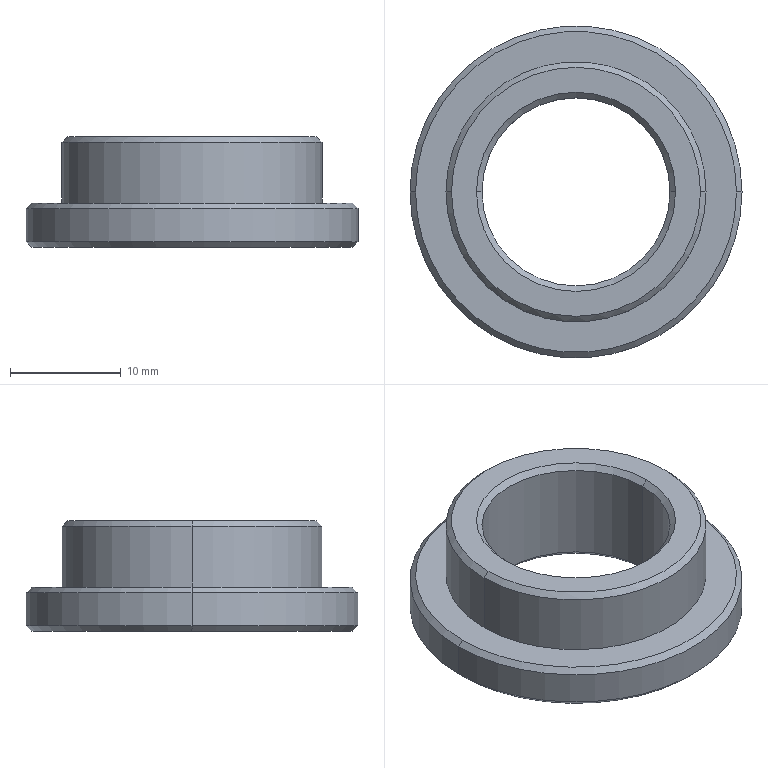Part | SolidWorks | features Chamfer 2, ICE 2, Extrusion 1 | 1 solid | 19 faces | box 30 x 30 x 10 mm | volume 3114 mm3 | cone 10 | cylinder 6 | plane 3 | commonest cylinder face diameters 17 x2 23.5 x2 30 x2
STEP:
#1=CARTESIAN_POINT('',(11.25,0.,10.));
#2=VERTEX_POINT('',#1);
#3=CARTESIAN_POINT('',(-11.25,0.,10.));
#4=VERTEX_POINT('',#3);
#5=CARTESIAN_POINT('',(0.,0.,10.));
#6=DIRECTION('',(0.,0.,1.));
#7=DIRECTION('',(1.,0.,0.));
#8=AXIS2_PLACEMENT_3D('',#5,#6,#7);
#9=CIRCLE('',#8,11.25);
#10=EDGE_CURVE('',#2,#4,#9,.T.);
#11=ORIENTED_EDGE('',*,*,#10,.F.);
#12=CARTESIAN_POINT('',(11.75,0.,9.5));
#13=VERTEX_POINT('',#12);
#14=CARTESIAN_POINT('',(11.25,0.,10.));
#15=DIRECTION('',(0.7071,0.,-0.7071));
#16=VECTOR('',#15,1000.);
#17=LINE('',#14,#16);
#18=EDGE_CURVE('',#2,#13,#17,.T.);
#19=ORIENTED_EDGE('',*,*,#18,.T.);
#20=CARTESIAN_POINT('',(-11.75,0.,9.5));
#21=VERTEX_POINT('',#20);
#22=CARTESIAN_POINT('',(0.,0.,9.5));
#23=DIRECTION('',(0.,0.,-1.));
#24=DIRECTION('',(1.,0.,0.));
#25=AXIS2_PLACEMENT_3D('',#22,#23,#24);
#26=CIRCLE('',#25,11.75);
#27=EDGE_CURVE('',#21,#13,#26,.T.);
#28=ORIENTED_EDGE('',*,*,#27,.F.);
#29=CARTESIAN_POINT('',(-11.25,0.,10.));
#30=DIRECTION('',(-0.7071,0.,-0.7071));
#31=VECTOR('',#30,1000.);
#32=LINE('',#29,#31);
#33=EDGE_CURVE('',#4,#21,#32,.T.);
#34=ORIENTED_EDGE('',*,*,#33,.F.);
#35=EDGE_LOOP('',(#11,#19,#28,#34));
#36=FACE_OUTER_BOUND('',#35,.T.);
#37=CARTESIAN_POINT('',(0.,0.,10.));
#38=DIRECTION('',(0.,0.,-1.));
#39=DIRECTION('',(-1.,0.,0.));
#40=AXIS2_PLACEMENT_3D('',#37,#38,#39);
#41=CONICAL_SURFACE('',#40,11.25,0.7854);
#42=ADVANCED_FACE('',(#36),#41,.T.);
#43=CARTESIAN_POINT('',(14.5,0.,4.));
#44=VERTEX_POINT('',#43);
#45=CARTESIAN_POINT('',(-14.5,0.,4.));
#46=VERTEX_POINT('',#45);
#47=CARTESIAN_POINT('',(0.,0.,4.));
#48=DIRECTION('',(0.,0.,1.));
#49=DIRECTION('',(1.,0.,0.));
#50=AXIS2_PLACEMENT_3D('',#47,#48,#49);
#51=CIRCLE('',#50,14.5);
#52=EDGE_CURVE('',#44,#46,#51,.T.);
#53=ORIENTED_EDGE('',*,*,#52,.F.);
#54=CARTESIAN_POINT('',(15.,0.,3.5));
#55=VERTEX_POINT('',#54);
#56=CARTESIAN_POINT('',(14.5,0.,4.));
#57=DIRECTION('',(0.7071,0.,-0.7071));
#58=VECTOR('',#57,1000.);
#59=LINE('',#56,#58);
#60=EDGE_CURVE('',#44,#55,#59,.T.);
#61=ORIENTED_EDGE('',*,*,#60,.T.);
#62=CARTESIAN_POINT('',(-15.,0.,3.5));
#63=VERTEX_POINT('',#62);
#64=CARTESIAN_POINT('',(0.,0.,3.5));
#65=DIRECTION('',(0.,0.,-1.));
#66=DIRECTION('',(1.,0.,0.));
#67=AXIS2_PLACEMENT_3D('',#64,#65,#66);
#68=CIRCLE('',#67,15.);
#69=EDGE_CURVE('',#63,#55,#68,.T.);
#70=ORIENTED_EDGE('',*,*,#69,.F.);
#71=CARTESIAN_POINT('',(-14.5,0.,4.));
#72=DIRECTION('',(-0.7071,0.,-0.7071));
#73=VECTOR('',#72,1000.);
#74=LINE('',#71,#73);
#75=EDGE_CURVE('',#46,#63,#74,.T.);
#76=ORIENTED_EDGE('',*,*,#75,.F.);
#77=EDGE_LOOP('',(#53,#61,#70,#76));
#78=FACE_OUTER_BOUND('',#77,.T.);
#79=CARTESIAN_POINT('',(0.,0.,4.));
#80=DIRECTION('',(0.,0.,-1.));
#81=DIRECTION('',(-1.,0.,0.));
#82=AXIS2_PLACEMENT_3D('',#79,#80,#81);
#83=CONICAL_SURFACE('',#82,14.5,0.7854);
#84=ADVANCED_FACE('',(#78),#83,.T.);
#85=CARTESIAN_POINT('',(-14.5,0.,0.));
#86=VERTEX_POINT('',#85);
#87=CARTESIAN_POINT('',(14.5,0.,0.));
#88=VERTEX_POINT('',#87);
#89=CARTESIAN_POINT('',(0.,0.,0.));
#90=DIRECTION('',(0.,0.,-1.));
#91=DIRECTION('',(1.,0.,0.));
#92=AXIS2_PLACEMENT_3D('',#89,#90,#91);
#93=CIRCLE('',#92,14.5);
#94=EDGE_CURVE('',#86,#88,#93,.T.);
#95=ORIENTED_EDGE('',*,*,#94,.F.);
#96=CARTESIAN_POINT('',(-15.,0.,0.5));
#97=VERTEX_POINT('',#96);
#98=CARTESIAN_POINT('',(-15.,0.,0.5));
#99=DIRECTION('',(-0.7071,0.,0.7071));
#100=VECTOR('',#99,1000.);
#101=LINE('',#98,#100);
#102=EDGE_CURVE('',#86,#97,#101,.T.);
#103=ORIENTED_EDGE('',*,*,#102,.T.);
#104=CARTESIAN_POINT('',(15.,0.,0.5));
#105=VERTEX_POINT('',#104);
#106=CARTESIAN_POINT('',(0.,0.,0.5));
#107=DIRECTION('',(0.,0.,1.));
#108=DIRECTION('',(1.,0.,0.));
#109=AXIS2_PLACEMENT_3D('',#106,#107,#108);
#110=CIRCLE('',#109,15.);
#111=EDGE_CURVE('',#105,#97,#110,.T.);
#112=ORIENTED_EDGE('',*,*,#111,.F.);
#113=CARTESIAN_POINT('',(15.,0.,0.5));
#114=DIRECTION('',(0.7071,0.,0.7071));
#115=VECTOR('',#114,1000.);
#116=LINE('',#113,#115);
#117=EDGE_CURVE('',#88,#105,#116,.T.);
#118=ORIENTED_EDGE('',*,*,#117,.F.);
#119=EDGE_LOOP('',(#95,#103,#112,#118));
#120=FACE_OUTER_BOUND('',#119,.T.);
#121=CARTESIAN_POINT('',(0.,0.,0.5));
#122=DIRECTION('',(0.,0.,1.));
#123=DIRECTION('',(1.,0.,0.));
#124=AXIS2_PLACEMENT_3D('',#121,#122,#123);
#125=CONICAL_SURFACE('',#124,15.,0.7854);
#126=ADVANCED_FACE('',(#120),#125,.T.);
#127=CARTESIAN_POINT('',(-8.5,0.,9.5));
#128=VERTEX_POINT('',#127);
#129=CARTESIAN_POINT('',(8.5,0.,9.5));
#130=VERTEX_POINT('',#129);
#131=CARTESIAN_POINT('',(0.,0.,9.5));
#132=DIRECTION('',(0.,0.,1.));
#133=DIRECTION('',(1.,0.,0.));
#134=AXIS2_PLACEMENT_3D('',#131,#132,#133);
#135=CIRCLE('',#134,8.5);
#136=EDGE_CURVE('',#128,#130,#135,.T.);
#137=ORIENTED_EDGE('',*,*,#136,.F.);
#138=CARTESIAN_POINT('',(-9.,0.,10.));
#139=VERTEX_POINT('',#138);
#140=CARTESIAN_POINT('',(-8.5,0.,9.5));
#141=DIRECTION('',(-0.7071,0.,0.7071));
#142=VECTOR('',#141,1000.);
#143=LINE('',#140,#142);
#144=EDGE_CURVE('',#128,#139,#143,.T.);
#145=ORIENTED_EDGE('',*,*,#144,.T.);
#146=CARTESIAN_POINT('',(9.,0.,10.));
#147=VERTEX_POINT('',#146);
#148=CARTESIAN_POINT('',(0.,0.,10.));
#149=DIRECTION('',(0.,0.,-1.));
#150=DIRECTION('',(1.,0.,0.));
#151=AXIS2_PLACEMENT_3D('',#148,#149,#150);
#152=CIRCLE('',#151,9.);
#153=EDGE_CURVE('',#147,#139,#152,.T.);
#154=ORIENTED_EDGE('',*,*,#153,.F.);
#155=CARTESIAN_POINT('',(8.5,0.,9.5));
#156=DIRECTION('',(0.7071,0.,0.7071));
#157=VECTOR('',#156,1000.);
#158=LINE('',#155,#157);
#159=EDGE_CURVE('',#130,#147,#158,.T.);
#160=ORIENTED_EDGE('',*,*,#159,.F.);
#161=EDGE_LOOP('',(#137,#145,#154,#160));
#162=FACE_OUTER_BOUND('',#161,.T.);
#163=CARTESIAN_POINT('',(0.,0.,9.5));
#164=DIRECTION('',(0.,0.,1.));
#165=DIRECTION('',(1.,0.,0.));
#166=AXIS2_PLACEMENT_3D('',#163,#164,#165);
#167=CONICAL_SURFACE('',#166,8.5,0.7854);
#168=ADVANCED_FACE('',(#162),#167,.F.);
#169=CARTESIAN_POINT('',(8.5,0.,0.5));
#170=VERTEX_POINT('',#169);
#171=CARTESIAN_POINT('',(-8.5,0.,0.5));
#172=VERTEX_POINT('',#171);
#173=CARTESIAN_POINT('',(0.,0.,0.5));
#174=DIRECTION('',(0.,0.,-1.));
#175=DIRECTION('',(1.,0.,0.));
#176=AXIS2_PLACEMENT_3D('',#173,#174,#175);
#177=CIRCLE('',#176,8.5);
#178=EDGE_CURVE('',#170,#172,#177,.T.);
#179=ORIENTED_EDGE('',*,*,#178,.F.);
#180=CARTESIAN_POINT('',(9.,0.,0.));
#181=VERTEX_POINT('',#180);
#182=CARTESIAN_POINT('',(8.5,0.,0.5));
#183=DIRECTION('',(0.7071,0.,-0.7071));
#184=VECTOR('',#183,1000.);
#185=LINE('',#182,#184);
#186=EDGE_CURVE('',#170,#181,#185,.T.);
#187=ORIENTED_EDGE('',*,*,#186,.T.);
#188=CARTESIAN_POINT('',(-9.,0.,0.));
#189=VERTEX_POINT('',#188);
#190=CARTESIAN_POINT('',(0.,0.,0.));
#191=DIRECTION('',(0.,0.,1.));
#192=DIRECTION('',(1.,0.,0.));
#193=AXIS2_PLACEMENT_3D('',#190,#191,#192);
#194=CIRCLE('',#193,9.);
#195=EDGE_CURVE('',#189,#181,#194,.T.);
#196=ORIENTED_EDGE('',*,*,#195,.F.);
#197=CARTESIAN_POINT('',(-8.5,0.,0.5));
#198=DIRECTION('',(-0.7071,0.,-0.7071));
#199=VECTOR('',#198,1000.);
#200=LINE('',#197,#199);
#201=EDGE_CURVE('',#172,#189,#200,.T.);
#202=ORIENTED_EDGE('',*,*,#201,.F.);
#203=EDGE_LOOP('',(#179,#187,#196,#202));
#204=FACE_OUTER_BOUND('',#203,.T.);
#205=CARTESIAN_POINT('',(0.,0.,0.5));
#206=DIRECTION('',(0.,0.,-1.));
#207=DIRECTION('',(-1.,0.,0.));
#208=AXIS2_PLACEMENT_3D('',#205,#206,#207);
#209=CONICAL_SURFACE('',#208,8.5,0.7854);
#210=ADVANCED_FACE('',(#204),#209,.F.);
#211=ORIENTED_EDGE('',*,*,#136,.T.);
#212=CARTESIAN_POINT('',(8.5,0.,20.));
#213=DIRECTION('',(0.,0.,-1.));
#214=VECTOR('',#213,1000.);
#215=LINE('',#212,#214);
#216=EDGE_CURVE('',#130,#170,#215,.T.);
#217=ORIENTED_EDGE('',*,*,#216,.T.);
#218=ORIENTED_EDGE('',*,*,#178,.T.);
#219=CARTESIAN_POINT('',(-8.5,0.,20.));
#220=DIRECTION('',(0.,0.,-1.));
#221=VECTOR('',#220,1000.);
#222=LINE('',#219,#221);
#223=EDGE_CURVE('',#128,#172,#222,.T.);
#224=ORIENTED_EDGE('',*,*,#223,.F.);
#225=EDGE_LOOP('',(#211,#217,#218,#224));
#226=FACE_OUTER_BOUND('',#225,.T.);
#227=CARTESIAN_POINT('',(0.,0.,20.));
#228=DIRECTION('',(0.,0.,-1.));
#229=DIRECTION('',(-1.,0.,0.));
#230=AXIS2_PLACEMENT_3D('',#227,#228,#229);
#231=CYLINDRICAL_SURFACE('',#230,8.5);
#232=ADVANCED_FACE('',(#226),#231,.F.);
#233=ORIENTED_EDGE('',*,*,#27,.T.);
#234=CARTESIAN_POINT('',(11.75,0.,4.));
#235=VERTEX_POINT('',#234);
#236=CARTESIAN_POINT('',(11.75,0.,10.));
#237=DIRECTION('',(0.,0.,-1.));
#238=VECTOR('',#237,1000.);
#239=LINE('',#236,#238);
#240=EDGE_CURVE('',#13,#235,#239,.T.);
#241=ORIENTED_EDGE('',*,*,#240,.T.);
#242=CARTESIAN_POINT('',(-11.75,0.,4.));
#243=VERTEX_POINT('',#242);
#244=CARTESIAN_POINT('',(0.,0.,4.));
#245=DIRECTION('',(0.,0.,1.));
#246=DIRECTION('',(1.,0.,0.));
#247=AXIS2_PLACEMENT_3D('',#244,#245,#246);
#248=CIRCLE('',#247,11.75);
#249=EDGE_CURVE('',#235,#243,#248,.T.);
#250=ORIENTED_EDGE('',*,*,#249,.T.);
#251=CARTESIAN_POINT('',(-11.75,0.,10.));
#252=DIRECTION('',(0.,0.,-1.));
#253=VECTOR('',#252,1000.);
#254=LINE('',#251,#253);
#255=EDGE_CURVE('',#21,#243,#254,.T.);
#256=ORIENTED_EDGE('',*,*,#255,.F.);
#257=EDGE_LOOP('',(#233,#241,#250,#256));
#258=FACE_OUTER_BOUND('',#257,.T.);
#259=CARTESIAN_POINT('',(0.,0.,10.));
#260=DIRECTION('',(0.,0.,-1.));
#261=DIRECTION('',(-1.,0.,0.));
#262=AXIS2_PLACEMENT_3D('',#259,#260,#261);
#263=CYLINDRICAL_SURFACE('',#262,11.75);
#264=ADVANCED_FACE('',(#258),#263,.T.);
#265=ORIENTED_EDGE('',*,*,#69,.T.);
#266=CARTESIAN_POINT('',(15.,0.,4.));
#267=DIRECTION('',(0.,0.,-1.));
#268=VECTOR('',#267,1000.);
#269=LINE('',#266,#268);
#270=EDGE_CURVE('',#55,#105,#269,.T.);
#271=ORIENTED_EDGE('',*,*,#270,.T.);
#272=ORIENTED_EDGE('',*,*,#111,.T.);
#273=CARTESIAN_POINT('',(-15.,0.,4.));
#274=DIRECTION('',(0.,0.,-1.));
#275=VECTOR('',#274,1000.);
#276=LINE('',#273,#275);
#277=EDGE_CURVE('',#63,#97,#276,.T.);
#278=ORIENTED_EDGE('',*,*,#277,.F.);
#279=EDGE_LOOP('',(#265,#271,#272,#278));
#280=FACE_OUTER_BOUND('',#279,.T.);
#281=CARTESIAN_POINT('',(0.,0.,4.));
#282=DIRECTION('',(0.,0.,-1.));
#283=DIRECTION('',(-1.,0.,0.));
#284=AXIS2_PLACEMENT_3D('',#281,#282,#283);
#285=CYLINDRICAL_SURFACE('',#284,15.);
#286=ADVANCED_FACE('',(#280),#285,.T.);
#287=ORIENTED_EDGE('',*,*,#270,.F.);
#288=CARTESIAN_POINT('',(0.,0.,3.5));
#289=DIRECTION('',(0.,0.,-1.));
#290=DIRECTION('',(1.,0.,0.));
#291=AXIS2_PLACEMENT_3D('',#288,#289,#290);
#292=CIRCLE('',#291,15.);
#293=EDGE_CURVE('',#55,#63,#292,.T.);
#294=ORIENTED_EDGE('',*,*,#293,.T.);
#295=ORIENTED_EDGE('',*,*,#277,.T.);
#296=CARTESIAN_POINT('',(0.,0.,0.5));
#297=DIRECTION('',(0.,0.,1.));
#298=DIRECTION('',(1.,0.,0.));
#299=AXIS2_PLACEMENT_3D('',#296,#297,#298);
#300=CIRCLE('',#299,15.);
#301=EDGE_CURVE('',#97,#105,#300,.T.);
#302=ORIENTED_EDGE('',*,*,#301,.T.);
#303=EDGE_LOOP('',(#287,#294,#295,#302));
#304=FACE_OUTER_BOUND('',#303,.T.);
#305=CARTESIAN_POINT('',(0.,0.,4.));
#306=DIRECTION('',(0.,0.,-1.));
#307=DIRECTION('',(-1.,0.,0.));
#308=AXIS2_PLACEMENT_3D('',#305,#306,#307);
#309=CYLINDRICAL_SURFACE('',#308,15.);
#310=ADVANCED_FACE('',(#304),#309,.T.);
#311=CARTESIAN_POINT('',(0.,0.,4.));
#312=DIRECTION('',(0.,0.,1.));
#313=DIRECTION('',(1.,0.,0.));
#314=AXIS2_PLACEMENT_3D('',#311,#312,#313);
#315=CIRCLE('',#314,14.5);
#316=EDGE_CURVE('',#46,#44,#315,.T.);
#317=ORIENTED_EDGE('',*,*,#316,.T.);
#318=ORIENTED_EDGE('',*,*,#52,.T.);
#319=EDGE_LOOP('',(#317,#318));
#320=FACE_OUTER_BOUND('',#319,.T.);
#321=CARTESIAN_POINT('',(0.,0.,4.));
#322=DIRECTION('',(0.,0.,1.));
#323=DIRECTION('',(1.,0.,0.));
#324=AXIS2_PLACEMENT_3D('',#321,#322,#323);
#325=CIRCLE('',#324,11.75);
#326=EDGE_CURVE('',#243,#235,#325,.T.);
#327=ORIENTED_EDGE('',*,*,#326,.F.);
#328=ORIENTED_EDGE('',*,*,#249,.F.);
#329=EDGE_LOOP('',(#327,#328));
#330=FACE_BOUND('',#329,.T.);
#331=CARTESIAN_POINT('',(0.,0.,4.));
#332=DIRECTION('',(0.,0.,1.));
#333=DIRECTION('',(1.,0.,0.));
#334=AXIS2_PLACEMENT_3D('',#331,#332,#333);
#335=PLANE('',#334);
#336=ADVANCED_FACE('',(#320,#330),#335,.T.);
#337=CARTESIAN_POINT('',(0.,0.,0.));
#338=DIRECTION('',(0.,0.,-1.));
#339=DIRECTION('',(1.,0.,0.));
#340=AXIS2_PLACEMENT_3D('',#337,#338,#339);
#341=CIRCLE('',#340,14.5);
#342=EDGE_CURVE('',#88,#86,#341,.T.);
#343=ORIENTED_EDGE('',*,*,#342,.T.);
#344=ORIENTED_EDGE('',*,*,#94,.T.);
#345=EDGE_LOOP('',(#343,#344));
#346=FACE_OUTER_BOUND('',#345,.T.);
#347=ORIENTED_EDGE('',*,*,#195,.T.);
#348=CARTESIAN_POINT('',(0.,0.,0.));
#349=DIRECTION('',(0.,0.,1.));
#350=DIRECTION('',(1.,0.,0.));
#351=AXIS2_PLACEMENT_3D('',#348,#349,#350);
#352=CIRCLE('',#351,9.);
#353=EDGE_CURVE('',#181,#189,#352,.T.);
#354=ORIENTED_EDGE('',*,*,#353,.T.);
#355=EDGE_LOOP('',(#347,#354));
#356=FACE_BOUND('',#355,.T.);
#357=CARTESIAN_POINT('',(0.,0.,0.));
#358=DIRECTION('',(0.,0.,1.));
#359=DIRECTION('',(1.,0.,0.));
#360=AXIS2_PLACEMENT_3D('',#357,#358,#359);
#361=PLANE('',#360);
#362=ADVANCED_FACE('',(#346,#356),#361,.F.);
#363=ORIENTED_EDGE('',*,*,#240,.F.);
#364=CARTESIAN_POINT('',(0.,0.,9.5));
#365=DIRECTION('',(0.,0.,-1.));
#366=DIRECTION('',(1.,0.,0.));
#367=AXIS2_PLACEMENT_3D('',#364,#365,#366);
#368=CIRCLE('',#367,11.75);
#369=EDGE_CURVE('',#13,#21,#368,.T.);
#370=ORIENTED_EDGE('',*,*,#369,.T.);
#371=ORIENTED_EDGE('',*,*,#255,.T.);
#372=ORIENTED_EDGE('',*,*,#326,.T.);
#373=EDGE_LOOP('',(#363,#370,#371,#372));
#374=FACE_OUTER_BOUND('',#373,.T.);
#375=CARTESIAN_POINT('',(0.,0.,10.));
#376=DIRECTION('',(0.,0.,-1.));
#377=DIRECTION('',(-1.,0.,0.));
#378=AXIS2_PLACEMENT_3D('',#375,#376,#377);
#379=CYLINDRICAL_SURFACE('',#378,11.75);
#380=ADVANCED_FACE('',(#374),#379,.T.);
#381=CARTESIAN_POINT('',(0.,0.,10.));
#382=DIRECTION('',(0.,0.,1.));
#383=DIRECTION('',(1.,0.,0.));
#384=AXIS2_PLACEMENT_3D('',#381,#382,#383);
#385=CIRCLE('',#384,11.25);
#386=EDGE_CURVE('',#4,#2,#385,.T.);
#387=ORIENTED_EDGE('',*,*,#386,.T.);
#388=ORIENTED_EDGE('',*,*,#10,.T.);
#389=EDGE_LOOP('',(#387,#388));
#390=FACE_OUTER_BOUND('',#389,.T.);
#391=ORIENTED_EDGE('',*,*,#153,.T.);
#392=CARTESIAN_POINT('',(0.,0.,10.));
#393=DIRECTION('',(0.,0.,-1.));
#394=DIRECTION('',(1.,0.,0.));
#395=AXIS2_PLACEMENT_3D('',#392,#393,#394);
#396=CIRCLE('',#395,9.);
#397=EDGE_CURVE('',#139,#147,#396,.T.);
#398=ORIENTED_EDGE('',*,*,#397,.T.);
#399=EDGE_LOOP('',(#391,#398));
#400=FACE_BOUND('',#399,.T.);
#401=CARTESIAN_POINT('',(0.,0.,10.));
#402=DIRECTION('',(0.,0.,1.));
#403=DIRECTION('',(1.,0.,0.));
#404=AXIS2_PLACEMENT_3D('',#401,#402,#403);
#405=PLANE('',#404);
#406=ADVANCED_FACE('',(#390,#400),#405,.T.);
#407=ORIENTED_EDGE('',*,*,#216,.F.);
#408=CARTESIAN_POINT('',(0.,0.,9.5));
#409=DIRECTION('',(0.,0.,1.));
#410=DIRECTION('',(1.,0.,0.));
#411=AXIS2_PLACEMENT_3D('',#408,#409,#410);
#412=CIRCLE('',#411,8.5);
#413=EDGE_CURVE('',#130,#128,#412,.T.);
#414=ORIENTED_EDGE('',*,*,#413,.T.);
#415=ORIENTED_EDGE('',*,*,#223,.T.);
#416=CARTESIAN_POINT('',(0.,0.,0.5));
#417=DIRECTION('',(0.,0.,-1.));
#418=DIRECTION('',(1.,0.,0.));
#419=AXIS2_PLACEMENT_3D('',#416,#417,#418);
#420=CIRCLE('',#419,8.5);
#421=EDGE_CURVE('',#172,#170,#420,.T.);
#422=ORIENTED_EDGE('',*,*,#421,.T.);
#423=EDGE_LOOP('',(#407,#414,#415,#422));
#424=FACE_OUTER_BOUND('',#423,.T.);
#425=CARTESIAN_POINT('',(0.,0.,20.));
#426=DIRECTION('',(0.,0.,-1.));
#427=DIRECTION('',(-1.,0.,0.));
#428=AXIS2_PLACEMENT_3D('',#425,#426,#427);
#429=CYLINDRICAL_SURFACE('',#428,8.5);
#430=ADVANCED_FACE('',(#424),#429,.F.);
#431=ORIENTED_EDGE('',*,*,#186,.F.);
#432=ORIENTED_EDGE('',*,*,#421,.F.);
#433=ORIENTED_EDGE('',*,*,#201,.T.);
#434=ORIENTED_EDGE('',*,*,#353,.F.);
#435=EDGE_LOOP('',(#431,#432,#433,#434));
#436=FACE_OUTER_BOUND('',#435,.T.);
#437=CARTESIAN_POINT('',(0.,0.,0.5));
#438=DIRECTION('',(0.,0.,-1.));
#439=DIRECTION('',(-1.,0.,0.));
#440=AXIS2_PLACEMENT_3D('',#437,#438,#439);
#441=CONICAL_SURFACE('',#440,8.5,0.7854);
#442=ADVANCED_FACE('',(#436),#441,.F.);
#443=ORIENTED_EDGE('',*,*,#144,.F.);
#444=ORIENTED_EDGE('',*,*,#413,.F.);
#445=ORIENTED_EDGE('',*,*,#159,.T.);
#446=ORIENTED_EDGE('',*,*,#397,.F.);
#447=EDGE_LOOP('',(#443,#444,#445,#446));
#448=FACE_OUTER_BOUND('',#447,.T.);
#449=CARTESIAN_POINT('',(0.,0.,9.5));
#450=DIRECTION('',(0.,0.,1.));
#451=DIRECTION('',(1.,0.,0.));
#452=AXIS2_PLACEMENT_3D('',#449,#450,#451);
#453=CONICAL_SURFACE('',#452,8.5,0.7854);
#454=ADVANCED_FACE('',(#448),#453,.F.);
#455=ORIENTED_EDGE('',*,*,#102,.F.);
#456=ORIENTED_EDGE('',*,*,#342,.F.);
#457=ORIENTED_EDGE('',*,*,#117,.T.);
#458=ORIENTED_EDGE('',*,*,#301,.F.);
#459=EDGE_LOOP('',(#455,#456,#457,#458));
#460=FACE_OUTER_BOUND('',#459,.T.);
#461=CARTESIAN_POINT('',(0.,0.,0.5));
#462=DIRECTION('',(0.,0.,1.));
#463=DIRECTION('',(1.,0.,0.));
#464=AXIS2_PLACEMENT_3D('',#461,#462,#463);
#465=CONICAL_SURFACE('',#464,15.,0.7854);
#466=ADVANCED_FACE('',(#460),#465,.T.);
#467=ORIENTED_EDGE('',*,*,#60,.F.);
#468=ORIENTED_EDGE('',*,*,#316,.F.);
#469=ORIENTED_EDGE('',*,*,#75,.T.);
#470=ORIENTED_EDGE('',*,*,#293,.F.);
#471=EDGE_LOOP('',(#467,#468,#469,#470));
#472=FACE_OUTER_BOUND('',#471,.T.);
#473=CARTESIAN_POINT('',(0.,0.,4.));
#474=DIRECTION('',(0.,0.,-1.));
#475=DIRECTION('',(-1.,0.,0.));
#476=AXIS2_PLACEMENT_3D('',#473,#474,#475);
#477=CONICAL_SURFACE('',#476,14.5,0.7854);
#478=ADVANCED_FACE('',(#472),#477,.T.);
#479=ORIENTED_EDGE('',*,*,#18,.F.);
#480=ORIENTED_EDGE('',*,*,#386,.F.);
#481=ORIENTED_EDGE('',*,*,#33,.T.);
#482=ORIENTED_EDGE('',*,*,#369,.F.);
#483=EDGE_LOOP('',(#479,#480,#481,#482));
#484=FACE_OUTER_BOUND('',#483,.T.);
#485=CARTESIAN_POINT('',(0.,0.,10.));
#486=DIRECTION('',(0.,0.,-1.));
#487=DIRECTION('',(-1.,0.,0.));
#488=AXIS2_PLACEMENT_3D('',#485,#486,#487);
#489=CONICAL_SURFACE('',#488,11.25,0.7854);
#490=ADVANCED_FACE('',(#484),#489,.T.);
#491=CLOSED_SHELL('',(#42,#84,#126,#168,#210,#232,#264,#286,#310,#336,#362,#380,#406,#430,#442,#454,#466,#478,#490));
#492=MANIFOLD_SOLID_BREP('',#491);
#493=CARTESIAN_POINT('',(0.,0.,0.));
#494=DIRECTION('',(0.,0.,1.));
#495=DIRECTION('',(1.,0.,0.));
#496=AXIS2_PLACEMENT_3D('',#493,#494,#495);
#497=(LENGTH_UNIT()NAMED_UNIT(*)SI_UNIT(.MILLI.,.METRE.));
#498=UNCERTAINTY_MEASURE_WITH_UNIT(LENGTH_MEASURE(0.00001),#497,'','');
#499=(NAMED_UNIT(*)PLANE_ANGLE_UNIT()SI_UNIT($,.RADIAN.));
#500=(NAMED_UNIT(*)SI_UNIT($,.STERADIAN.)SOLID_ANGLE_UNIT());
#501=(GEOMETRIC_REPRESENTATION_CONTEXT(3)GLOBAL_UNCERTAINTY_ASSIGNED_CONTEXT((#498))GLOBAL_UNIT_ASSIGNED_CONTEXT((#497,#499,#500))REPRESENTATION_CONTEXT('',''));
#502=ADVANCED_BREP_SHAPE_REPRESENTATION('',(#492,#496),#501);